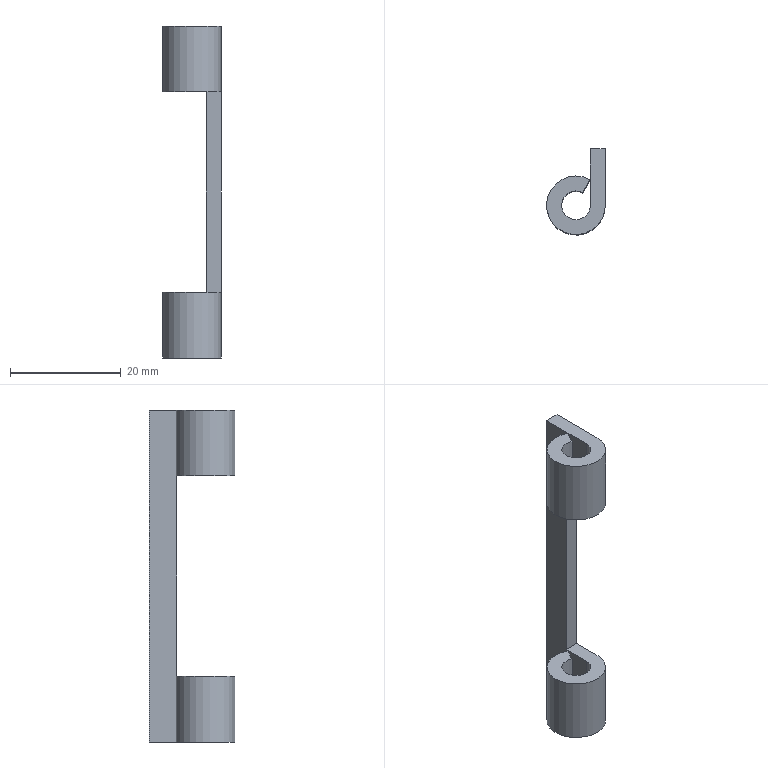Part | SolidWorks | features BaseBody 1 | 1 solid | 14 faces | box 10.6 x 15.5 x 60 mm | volume 2458 mm3 | plane 10 | cylinder 4 | commonest cylinder face diameters 5.2 x2 10.6 x2
STEP:
#1=CARTESIAN_POINT('',(2.6,10.2,-30.));
#2=VERTEX_POINT('',#1);
#3=CARTESIAN_POINT('',(2.6,10.2,30.));
#4=VERTEX_POINT('',#3);
#5=CARTESIAN_POINT('',(2.6,10.2,30.));
#6=DIRECTION('',(0.,0.,1.));
#7=VECTOR('',#6,1000.);
#8=LINE('',#5,#7);
#9=EDGE_CURVE('',#2,#4,#8,.T.);
#10=ORIENTED_EDGE('',*,*,#9,.F.);
#11=CARTESIAN_POINT('',(2.6,0.,-30.));
#12=VERTEX_POINT('',#11);
#13=CARTESIAN_POINT('',(2.6,10.2,-30.));
#14=DIRECTION('',(0.,1.,0.));
#15=VECTOR('',#14,1000.);
#16=LINE('',#13,#15);
#17=EDGE_CURVE('',#12,#2,#16,.T.);
#18=ORIENTED_EDGE('',*,*,#17,.F.);
#19=CARTESIAN_POINT('',(2.6,0.,-18.15));
#20=VERTEX_POINT('',#19);
#21=CARTESIAN_POINT('',(2.6,0.,30.));
#22=DIRECTION('',(0.,0.,-1.));
#23=VECTOR('',#22,1000.);
#24=LINE('',#21,#23);
#25=EDGE_CURVE('',#20,#12,#24,.T.);
#26=ORIENTED_EDGE('',*,*,#25,.F.);
#27=CARTESIAN_POINT('',(2.6,5.2,-18.15));
#28=VERTEX_POINT('',#27);
#29=CARTESIAN_POINT('',(2.6,10.2,-18.15));
#30=DIRECTION('',(0.,-1.,0.));
#31=VECTOR('',#30,1000.);
#32=LINE('',#29,#31);
#33=EDGE_CURVE('',#28,#20,#32,.T.);
#34=ORIENTED_EDGE('',*,*,#33,.F.);
#35=CARTESIAN_POINT('',(2.6,5.2,18.15));
#36=VERTEX_POINT('',#35);
#37=CARTESIAN_POINT('',(2.6,5.2,30.));
#38=DIRECTION('',(0.,0.,-1.));
#39=VECTOR('',#38,1000.);
#40=LINE('',#37,#39);
#41=EDGE_CURVE('',#36,#28,#40,.T.);
#42=ORIENTED_EDGE('',*,*,#41,.F.);
#43=CARTESIAN_POINT('',(2.6,0.,18.15));
#44=VERTEX_POINT('',#43);
#45=CARTESIAN_POINT('',(2.6,10.2,18.15));
#46=DIRECTION('',(0.,1.,0.));
#47=VECTOR('',#46,1000.);
#48=LINE('',#45,#47);
#49=EDGE_CURVE('',#44,#36,#48,.T.);
#50=ORIENTED_EDGE('',*,*,#49,.F.);
#51=CARTESIAN_POINT('',(2.6,0.,30.));
#52=VERTEX_POINT('',#51);
#53=CARTESIAN_POINT('',(2.6,0.,30.));
#54=DIRECTION('',(0.,0.,-1.));
#55=VECTOR('',#54,1000.);
#56=LINE('',#53,#55);
#57=EDGE_CURVE('',#52,#44,#56,.T.);
#58=ORIENTED_EDGE('',*,*,#57,.F.);
#59=CARTESIAN_POINT('',(2.6,10.2,30.));
#60=DIRECTION('',(0.,-1.,0.));
#61=VECTOR('',#60,1000.);
#62=LINE('',#59,#61);
#63=EDGE_CURVE('',#4,#52,#62,.T.);
#64=ORIENTED_EDGE('',*,*,#63,.F.);
#65=EDGE_LOOP('',(#10,#18,#26,#34,#42,#50,#58,#64));
#66=FACE_OUTER_BOUND('',#65,.T.);
#67=CARTESIAN_POINT('',(2.6,10.2,30.));
#68=DIRECTION('',(1.,0.,0.));
#69=DIRECTION('',(0.,0.,-1.));
#70=AXIS2_PLACEMENT_3D('',#67,#68,#69);
#71=PLANE('',#70);
#72=ADVANCED_FACE('',(#66),#71,.F.);
#73=CARTESIAN_POINT('',(1.229,2.291,30.));
#74=VERTEX_POINT('',#73);
#75=CARTESIAN_POINT('',(2.505,4.671,30.));
#76=VERTEX_POINT('',#75);
#77=CARTESIAN_POINT('',(1.229,2.291,30.));
#78=DIRECTION('',(0.4726,0.8813,0.));
#79=VECTOR('',#78,1000.);
#80=LINE('',#77,#79);
#81=EDGE_CURVE('',#74,#76,#80,.T.);
#82=ORIENTED_EDGE('',*,*,#81,.T.);
#83=CARTESIAN_POINT('',(5.3,0.,30.));
#84=VERTEX_POINT('',#83);
#85=CARTESIAN_POINT('',(0.,0.,30.));
#86=DIRECTION('',(0.,0.,1.));
#87=DIRECTION('',(1.,0.,0.));
#88=AXIS2_PLACEMENT_3D('',#85,#86,#87);
#89=CIRCLE('',#88,5.3);
#90=EDGE_CURVE('',#76,#84,#89,.T.);
#91=ORIENTED_EDGE('',*,*,#90,.T.);
#92=CARTESIAN_POINT('',(5.3,10.2,30.));
#93=VERTEX_POINT('',#92);
#94=CARTESIAN_POINT('',(5.3,0.,30.));
#95=DIRECTION('',(0.,1.,0.));
#96=VECTOR('',#95,1000.);
#97=LINE('',#94,#96);
#98=EDGE_CURVE('',#84,#93,#97,.T.);
#99=ORIENTED_EDGE('',*,*,#98,.T.);
#100=CARTESIAN_POINT('',(0.,10.2,30.));
#101=DIRECTION('',(-1.,0.,0.));
#102=VECTOR('',#101,1000.);
#103=LINE('',#100,#102);
#104=EDGE_CURVE('',#93,#4,#103,.T.);
#105=ORIENTED_EDGE('',*,*,#104,.T.);
#106=ORIENTED_EDGE('',*,*,#63,.T.);
#107=CARTESIAN_POINT('',(0.,0.,30.));
#108=DIRECTION('',(0.,0.,-1.));
#109=DIRECTION('',(1.,0.,0.));
#110=AXIS2_PLACEMENT_3D('',#107,#108,#109);
#111=CIRCLE('',#110,2.6);
#112=EDGE_CURVE('',#52,#74,#111,.T.);
#113=ORIENTED_EDGE('',*,*,#112,.T.);
#114=EDGE_LOOP('',(#82,#91,#99,#105,#106,#113));
#115=FACE_OUTER_BOUND('',#114,.T.);
#116=CARTESIAN_POINT('',(0.,0.,30.));
#117=DIRECTION('',(0.,0.,1.));
#118=DIRECTION('',(1.,0.,0.));
#119=AXIS2_PLACEMENT_3D('',#116,#117,#118);
#120=PLANE('',#119);
#121=ADVANCED_FACE('',(#115),#120,.T.);
#122=ORIENTED_EDGE('',*,*,#104,.F.);
#123=CARTESIAN_POINT('',(5.3,10.2,-30.));
#124=VERTEX_POINT('',#123);
#125=CARTESIAN_POINT('',(5.3,10.2,0.));
#126=DIRECTION('',(0.,0.,1.));
#127=VECTOR('',#126,1000.);
#128=LINE('',#125,#127);
#129=EDGE_CURVE('',#124,#93,#128,.T.);
#130=ORIENTED_EDGE('',*,*,#129,.F.);
#131=CARTESIAN_POINT('',(0.,10.2,-30.));
#132=DIRECTION('',(1.,0.,0.));
#133=VECTOR('',#132,1000.);
#134=LINE('',#131,#133);
#135=EDGE_CURVE('',#2,#124,#134,.T.);
#136=ORIENTED_EDGE('',*,*,#135,.F.);
#137=ORIENTED_EDGE('',*,*,#9,.T.);
#138=EDGE_LOOP('',(#122,#130,#136,#137));
#139=FACE_OUTER_BOUND('',#138,.T.);
#140=CARTESIAN_POINT('',(0.,10.2,0.));
#141=DIRECTION('',(0.,-1.,0.));
#142=DIRECTION('',(0.,0.,-1.));
#143=AXIS2_PLACEMENT_3D('',#140,#141,#142);
#144=PLANE('',#143);
#145=ADVANCED_FACE('',(#139),#144,.F.);
#146=CARTESIAN_POINT('',(2.505,4.671,-30.));
#147=VERTEX_POINT('',#146);
#148=CARTESIAN_POINT('',(1.229,2.291,-30.));
#149=VERTEX_POINT('',#148);
#150=CARTESIAN_POINT('',(2.505,4.671,-30.));
#151=DIRECTION('',(-0.4726,-0.8813,0.));
#152=VECTOR('',#151,1000.);
#153=LINE('',#150,#152);
#154=EDGE_CURVE('',#147,#149,#153,.T.);
#155=ORIENTED_EDGE('',*,*,#154,.T.);
#156=CARTESIAN_POINT('',(0.,0.,-30.));
#157=DIRECTION('',(0.,0.,1.));
#158=DIRECTION('',(1.,0.,0.));
#159=AXIS2_PLACEMENT_3D('',#156,#157,#158);
#160=CIRCLE('',#159,2.6);
#161=EDGE_CURVE('',#149,#12,#160,.T.);
#162=ORIENTED_EDGE('',*,*,#161,.T.);
#163=ORIENTED_EDGE('',*,*,#17,.T.);
#164=ORIENTED_EDGE('',*,*,#135,.T.);
#165=CARTESIAN_POINT('',(5.3,0.,-30.));
#166=VERTEX_POINT('',#165);
#167=CARTESIAN_POINT('',(5.3,0.,-30.));
#168=DIRECTION('',(0.,-1.,0.));
#169=VECTOR('',#168,1000.);
#170=LINE('',#167,#169);
#171=EDGE_CURVE('',#124,#166,#170,.T.);
#172=ORIENTED_EDGE('',*,*,#171,.T.);
#173=CARTESIAN_POINT('',(0.,0.,-30.));
#174=DIRECTION('',(0.,0.,-1.));
#175=DIRECTION('',(1.,0.,0.));
#176=AXIS2_PLACEMENT_3D('',#173,#174,#175);
#177=CIRCLE('',#176,5.3);
#178=EDGE_CURVE('',#166,#147,#177,.T.);
#179=ORIENTED_EDGE('',*,*,#178,.T.);
#180=EDGE_LOOP('',(#155,#162,#163,#164,#172,#179));
#181=FACE_OUTER_BOUND('',#180,.T.);
#182=CARTESIAN_POINT('',(0.,0.,-30.));
#183=DIRECTION('',(0.,0.,-1.));
#184=DIRECTION('',(-1.,0.,0.));
#185=AXIS2_PLACEMENT_3D('',#182,#183,#184);
#186=PLANE('',#185);
#187=ADVANCED_FACE('',(#181),#186,.T.);
#188=ORIENTED_EDGE('',*,*,#25,.T.);
#189=ORIENTED_EDGE('',*,*,#161,.F.);
#190=CARTESIAN_POINT('',(1.229,2.291,-18.15));
#191=VERTEX_POINT('',#190);
#192=CARTESIAN_POINT('',(1.229,2.291,-30.));
#193=DIRECTION('',(0.,0.,-1.));
#194=VECTOR('',#193,1000.);
#195=LINE('',#192,#194);
#196=EDGE_CURVE('',#191,#149,#195,.T.);
#197=ORIENTED_EDGE('',*,*,#196,.F.);
#198=CARTESIAN_POINT('',(0.,0.,-18.15));
#199=DIRECTION('',(0.,0.,-1.));
#200=DIRECTION('',(1.,0.,0.));
#201=AXIS2_PLACEMENT_3D('',#198,#199,#200);
#202=CIRCLE('',#201,2.6);
#203=EDGE_CURVE('',#20,#191,#202,.T.);
#204=ORIENTED_EDGE('',*,*,#203,.F.);
#205=EDGE_LOOP('',(#188,#189,#197,#204));
#206=FACE_OUTER_BOUND('',#205,.T.);
#207=CARTESIAN_POINT('',(0.,0.,-30.));
#208=DIRECTION('',(0.,0.,1.));
#209=DIRECTION('',(1.,0.,0.));
#210=AXIS2_PLACEMENT_3D('',#207,#208,#209);
#211=CYLINDRICAL_SURFACE('',#210,2.6);
#212=ADVANCED_FACE('',(#206),#211,.F.);
#213=CARTESIAN_POINT('',(5.3,5.2,-18.15));
#214=VERTEX_POINT('',#213);
#215=CARTESIAN_POINT('',(0.,5.2,-18.15));
#216=DIRECTION('',(1.,0.,0.));
#217=VECTOR('',#216,1000.);
#218=LINE('',#215,#217);
#219=EDGE_CURVE('',#28,#214,#218,.T.);
#220=ORIENTED_EDGE('',*,*,#219,.F.);
#221=ORIENTED_EDGE('',*,*,#33,.T.);
#222=ORIENTED_EDGE('',*,*,#203,.T.);
#223=CARTESIAN_POINT('',(2.505,4.671,-18.15));
#224=VERTEX_POINT('',#223);
#225=CARTESIAN_POINT('',(2.505,4.671,-18.15));
#226=DIRECTION('',(-0.4726,-0.8813,0.));
#227=VECTOR('',#226,1000.);
#228=LINE('',#225,#227);
#229=EDGE_CURVE('',#224,#191,#228,.T.);
#230=ORIENTED_EDGE('',*,*,#229,.F.);
#231=CARTESIAN_POINT('',(5.3,0.,-18.15));
#232=VERTEX_POINT('',#231);
#233=CARTESIAN_POINT('',(0.,0.,-18.15));
#234=DIRECTION('',(0.,0.,-1.));
#235=DIRECTION('',(1.,0.,0.));
#236=AXIS2_PLACEMENT_3D('',#233,#234,#235);
#237=CIRCLE('',#236,5.3);
#238=EDGE_CURVE('',#232,#224,#237,.T.);
#239=ORIENTED_EDGE('',*,*,#238,.F.);
#240=CARTESIAN_POINT('',(5.3,0.,-18.15));
#241=DIRECTION('',(0.,-1.,0.));
#242=VECTOR('',#241,1000.);
#243=LINE('',#240,#242);
#244=EDGE_CURVE('',#214,#232,#243,.T.);
#245=ORIENTED_EDGE('',*,*,#244,.F.);
#246=EDGE_LOOP('',(#220,#221,#222,#230,#239,#245));
#247=FACE_OUTER_BOUND('',#246,.T.);
#248=CARTESIAN_POINT('',(0.,0.,-18.15));
#249=DIRECTION('',(0.,0.,-1.));
#250=DIRECTION('',(-1.,0.,0.));
#251=AXIS2_PLACEMENT_3D('',#248,#249,#250);
#252=PLANE('',#251);
#253=ADVANCED_FACE('',(#247),#252,.F.);
#254=ORIENTED_EDGE('',*,*,#41,.T.);
#255=ORIENTED_EDGE('',*,*,#219,.T.);
#256=CARTESIAN_POINT('',(5.3,5.2,18.15));
#257=VERTEX_POINT('',#256);
#258=CARTESIAN_POINT('',(5.3,5.2,-18.15));
#259=DIRECTION('',(0.,0.,-1.));
#260=VECTOR('',#259,1000.);
#261=LINE('',#258,#260);
#262=EDGE_CURVE('',#257,#214,#261,.T.);
#263=ORIENTED_EDGE('',*,*,#262,.F.);
#264=CARTESIAN_POINT('',(2.6,5.2,18.15));
#265=DIRECTION('',(1.,0.,0.));
#266=VECTOR('',#265,1000.);
#267=LINE('',#264,#266);
#268=EDGE_CURVE('',#36,#257,#267,.T.);
#269=ORIENTED_EDGE('',*,*,#268,.F.);
#270=EDGE_LOOP('',(#254,#255,#263,#269));
#271=FACE_OUTER_BOUND('',#270,.T.);
#272=CARTESIAN_POINT('',(2.6,5.2,-18.15));
#273=DIRECTION('',(0.,1.,0.));
#274=DIRECTION('',(0.,0.,1.));
#275=AXIS2_PLACEMENT_3D('',#272,#273,#274);
#276=PLANE('',#275);
#277=ADVANCED_FACE('',(#271),#276,.F.);
#278=CARTESIAN_POINT('',(1.229,2.291,18.15));
#279=VERTEX_POINT('',#278);
#280=CARTESIAN_POINT('',(0.,0.,18.15));
#281=DIRECTION('',(0.,0.,1.));
#282=DIRECTION('',(1.,0.,0.));
#283=AXIS2_PLACEMENT_3D('',#280,#281,#282);
#284=CIRCLE('',#283,2.6);
#285=EDGE_CURVE('',#279,#44,#284,.T.);
#286=ORIENTED_EDGE('',*,*,#285,.T.);
#287=ORIENTED_EDGE('',*,*,#49,.T.);
#288=ORIENTED_EDGE('',*,*,#268,.T.);
#289=CARTESIAN_POINT('',(5.3,0.,18.15));
#290=VERTEX_POINT('',#289);
#291=CARTESIAN_POINT('',(5.3,6.,18.15));
#292=DIRECTION('',(0.,-1.,0.));
#293=VECTOR('',#292,1000.);
#294=LINE('',#291,#293);
#295=EDGE_CURVE('',#257,#290,#294,.T.);
#296=ORIENTED_EDGE('',*,*,#295,.T.);
#297=CARTESIAN_POINT('',(2.505,4.671,18.15));
#298=VERTEX_POINT('',#297);
#299=CARTESIAN_POINT('',(0.,0.,18.15));
#300=DIRECTION('',(0.,0.,-1.));
#301=DIRECTION('',(1.,0.,0.));
#302=AXIS2_PLACEMENT_3D('',#299,#300,#301);
#303=CIRCLE('',#302,5.3);
#304=EDGE_CURVE('',#290,#298,#303,.T.);
#305=ORIENTED_EDGE('',*,*,#304,.T.);
#306=CARTESIAN_POINT('',(2.505,4.671,18.15));
#307=DIRECTION('',(-0.4726,-0.8813,0.));
#308=VECTOR('',#307,1000.);
#309=LINE('',#306,#308);
#310=EDGE_CURVE('',#298,#279,#309,.T.);
#311=ORIENTED_EDGE('',*,*,#310,.T.);
#312=EDGE_LOOP('',(#286,#287,#288,#296,#305,#311));
#313=FACE_OUTER_BOUND('',#312,.T.);
#314=CARTESIAN_POINT('',(-7.4,6.,18.15));
#315=DIRECTION('',(0.,0.,-1.));
#316=DIRECTION('',(-1.,0.,0.));
#317=AXIS2_PLACEMENT_3D('',#314,#315,#316);
#318=PLANE('',#317);
#319=ADVANCED_FACE('',(#313),#318,.T.);
#320=ORIENTED_EDGE('',*,*,#285,.F.);
#321=CARTESIAN_POINT('',(1.229,2.291,30.));
#322=DIRECTION('',(0.,0.,1.));
#323=VECTOR('',#322,1000.);
#324=LINE('',#321,#323);
#325=EDGE_CURVE('',#279,#74,#324,.T.);
#326=ORIENTED_EDGE('',*,*,#325,.T.);
#327=ORIENTED_EDGE('',*,*,#112,.F.);
#328=ORIENTED_EDGE('',*,*,#57,.T.);
#329=EDGE_LOOP('',(#320,#326,#327,#328));
#330=FACE_OUTER_BOUND('',#329,.T.);
#331=CARTESIAN_POINT('',(0.,0.,30.));
#332=DIRECTION('',(0.,0.,1.));
#333=DIRECTION('',(1.,0.,0.));
#334=AXIS2_PLACEMENT_3D('',#331,#332,#333);
#335=CYLINDRICAL_SURFACE('',#334,2.6);
#336=ADVANCED_FACE('',(#330),#335,.F.);
#337=CARTESIAN_POINT('',(5.3,0.,30.));
#338=DIRECTION('',(0.,0.,1.));
#339=VECTOR('',#338,1000.);
#340=LINE('',#337,#339);
#341=EDGE_CURVE('',#290,#84,#340,.T.);
#342=ORIENTED_EDGE('',*,*,#341,.T.);
#343=ORIENTED_EDGE('',*,*,#90,.F.);
#344=CARTESIAN_POINT('',(2.505,4.671,30.));
#345=DIRECTION('',(0.,0.,-1.));
#346=VECTOR('',#345,1000.);
#347=LINE('',#344,#346);
#348=EDGE_CURVE('',#76,#298,#347,.T.);
#349=ORIENTED_EDGE('',*,*,#348,.T.);
#350=ORIENTED_EDGE('',*,*,#304,.F.);
#351=EDGE_LOOP('',(#342,#343,#349,#350));
#352=FACE_OUTER_BOUND('',#351,.T.);
#353=CARTESIAN_POINT('',(0.,0.,30.));
#354=DIRECTION('',(0.,0.,1.));
#355=DIRECTION('',(1.,0.,0.));
#356=AXIS2_PLACEMENT_3D('',#353,#354,#355);
#357=CYLINDRICAL_SURFACE('',#356,5.3);
#358=ADVANCED_FACE('',(#352),#357,.T.);
#359=ORIENTED_EDGE('',*,*,#348,.F.);
#360=ORIENTED_EDGE('',*,*,#81,.F.);
#361=ORIENTED_EDGE('',*,*,#325,.F.);
#362=ORIENTED_EDGE('',*,*,#310,.F.);
#363=EDGE_LOOP('',(#359,#360,#361,#362));
#364=FACE_OUTER_BOUND('',#363,.T.);
#365=CARTESIAN_POINT('',(1.229,2.291,30.));
#366=DIRECTION('',(-0.8813,0.4726,0.));
#367=DIRECTION('',(-0.4726,-0.8813,0.));
#368=AXIS2_PLACEMENT_3D('',#365,#366,#367);
#369=PLANE('',#368);
#370=ADVANCED_FACE('',(#364),#369,.F.);
#371=ORIENTED_EDGE('',*,*,#98,.F.);
#372=ORIENTED_EDGE('',*,*,#341,.F.);
#373=ORIENTED_EDGE('',*,*,#295,.F.);
#374=ORIENTED_EDGE('',*,*,#262,.T.);
#375=ORIENTED_EDGE('',*,*,#244,.T.);
#376=CARTESIAN_POINT('',(5.3,0.,30.));
#377=DIRECTION('',(0.,0.,-1.));
#378=VECTOR('',#377,1000.);
#379=LINE('',#376,#378);
#380=EDGE_CURVE('',#232,#166,#379,.T.);
#381=ORIENTED_EDGE('',*,*,#380,.T.);
#382=ORIENTED_EDGE('',*,*,#171,.F.);
#383=ORIENTED_EDGE('',*,*,#129,.T.);
#384=EDGE_LOOP('',(#371,#372,#373,#374,#375,#381,#382,#383));
#385=FACE_OUTER_BOUND('',#384,.T.);
#386=CARTESIAN_POINT('',(5.3,2.599,30.));
#387=DIRECTION('',(1.,0.,0.));
#388=DIRECTION('',(0.,1.,0.));
#389=AXIS2_PLACEMENT_3D('',#386,#387,#388);
#390=PLANE('',#389);
#391=ADVANCED_FACE('',(#385),#390,.T.);
#392=ORIENTED_EDGE('',*,*,#196,.T.);
#393=ORIENTED_EDGE('',*,*,#154,.F.);
#394=CARTESIAN_POINT('',(2.505,4.671,-30.));
#395=DIRECTION('',(0.,0.,-1.));
#396=VECTOR('',#395,1000.);
#397=LINE('',#394,#396);
#398=EDGE_CURVE('',#224,#147,#397,.T.);
#399=ORIENTED_EDGE('',*,*,#398,.F.);
#400=ORIENTED_EDGE('',*,*,#229,.T.);
#401=EDGE_LOOP('',(#392,#393,#399,#400));
#402=FACE_OUTER_BOUND('',#401,.T.);
#403=CARTESIAN_POINT('',(1.229,2.291,-30.));
#404=DIRECTION('',(-0.8813,0.4726,0.));
#405=DIRECTION('',(-0.4726,-0.8813,0.));
#406=AXIS2_PLACEMENT_3D('',#403,#404,#405);
#407=PLANE('',#406);
#408=ADVANCED_FACE('',(#402),#407,.F.);
#409=ORIENTED_EDGE('',*,*,#178,.F.);
#410=ORIENTED_EDGE('',*,*,#380,.F.);
#411=ORIENTED_EDGE('',*,*,#238,.T.);
#412=ORIENTED_EDGE('',*,*,#398,.T.);
#413=EDGE_LOOP('',(#409,#410,#411,#412));
#414=FACE_OUTER_BOUND('',#413,.T.);
#415=CARTESIAN_POINT('',(0.,0.,-30.));
#416=DIRECTION('',(0.,0.,1.));
#417=DIRECTION('',(1.,0.,0.));
#418=AXIS2_PLACEMENT_3D('',#415,#416,#417);
#419=CYLINDRICAL_SURFACE('',#418,5.3);
#420=ADVANCED_FACE('',(#414),#419,.T.);
#421=CLOSED_SHELL('',(#72,#121,#145,#187,#212,#253,#277,#319,#336,#358,#370,#391,#408,#420));
#422=MANIFOLD_SOLID_BREP('',#421);
#423=CARTESIAN_POINT('',(0.,0.,0.));
#424=DIRECTION('',(0.,0.,1.));
#425=DIRECTION('',(1.,0.,0.));
#426=AXIS2_PLACEMENT_3D('',#423,#424,#425);
#427=(LENGTH_UNIT()NAMED_UNIT(*)SI_UNIT(.MILLI.,.METRE.));
#428=UNCERTAINTY_MEASURE_WITH_UNIT(LENGTH_MEASURE(0.00001),#427,'','');
#429=(NAMED_UNIT(*)PLANE_ANGLE_UNIT()SI_UNIT($,.RADIAN.));
#430=(NAMED_UNIT(*)SI_UNIT($,.STERADIAN.)SOLID_ANGLE_UNIT());
#431=(GEOMETRIC_REPRESENTATION_CONTEXT(3)GLOBAL_UNCERTAINTY_ASSIGNED_CONTEXT((#428))GLOBAL_UNIT_ASSIGNED_CONTEXT((#427,#429,#430))REPRESENTATION_CONTEXT('',''));
#432=ADVANCED_BREP_SHAPE_REPRESENTATION('',(#422,#426),#431);